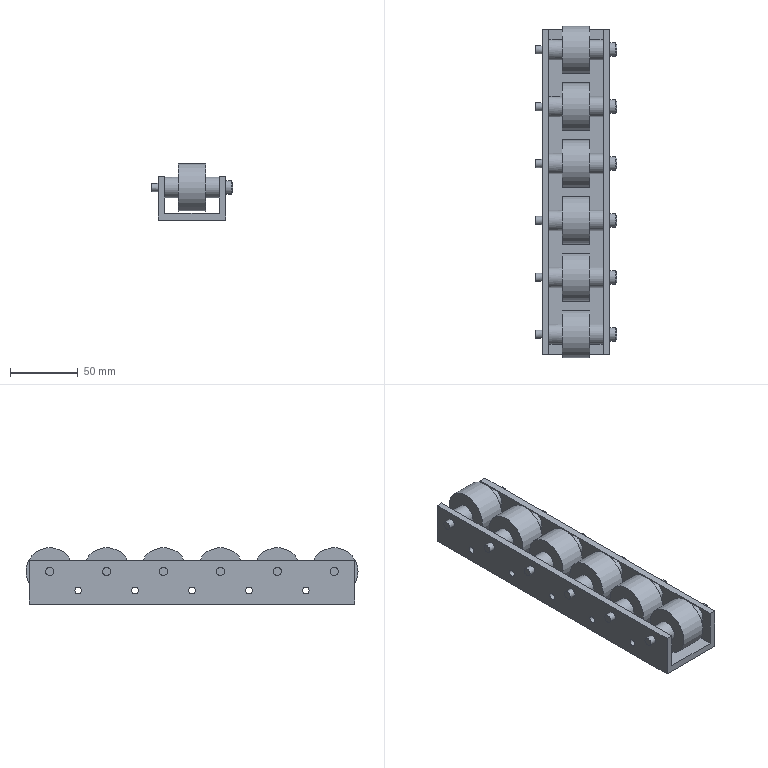Part | NX | features solid 2 | 1 solid | 80 faces | box 60 x 245 x 41.5 mm | volume 263594 mm3 | cylinder 40 | plane 34 | cone 6 | commonest cylinder face diameters 15 x12 5 x10 6 x6 10 x6 35 x6